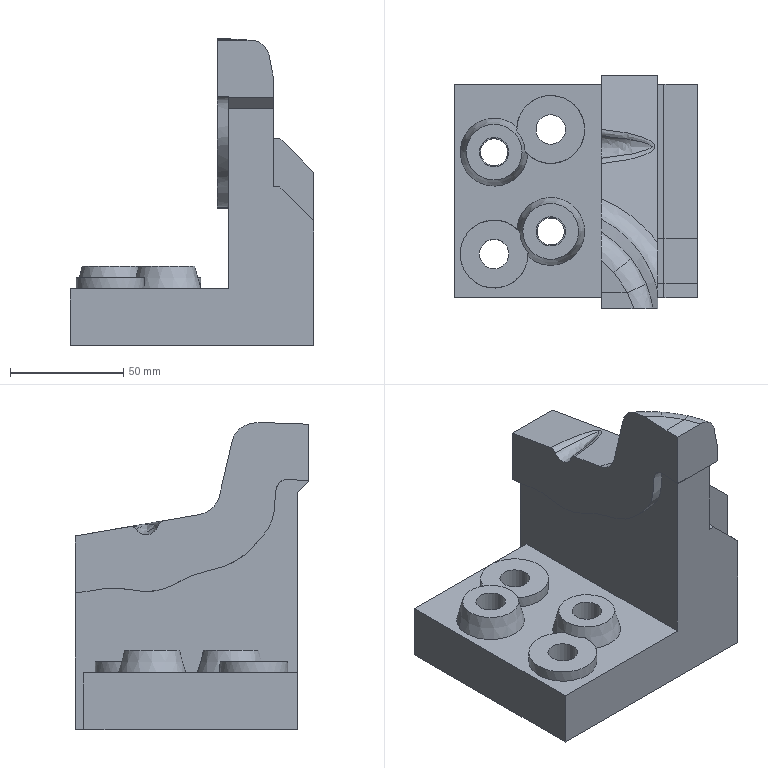Part | NX | features solid 2 | 1 solid | 48 faces | box 107.683 x 103.154 x 135.702 mm | volume 495592 mm3 | plane 27 | spline 11 | cylinder 8 | cone 2 | commonest cylinder face diameters 13 x4 12 x2 30 x2